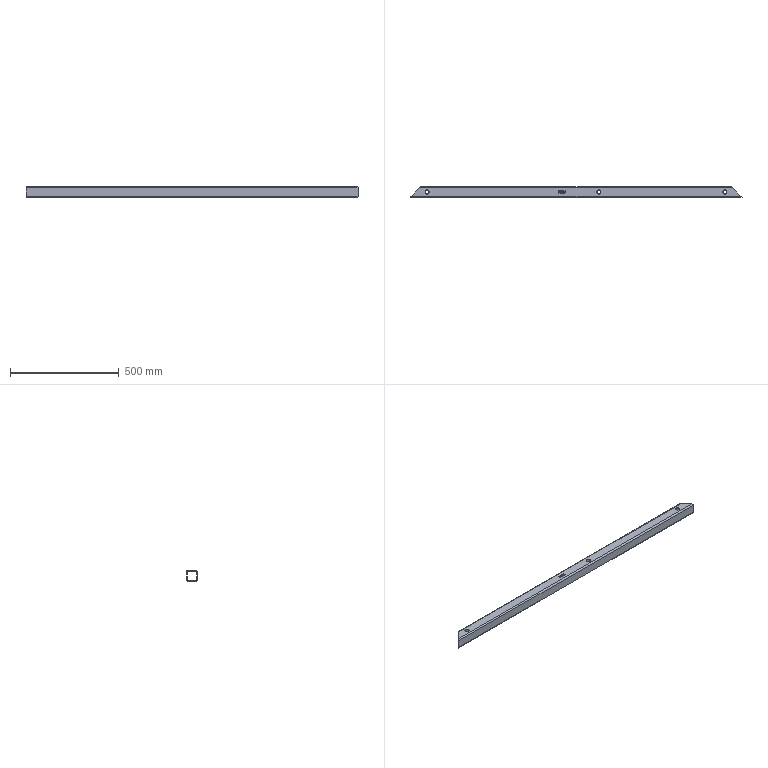Part | SolidWorks | features BaseBody 1 | 1 solid | 118 faces | box 1527 x 50 x 50 mm | volume 794723 mm3 | plane 68 | spline 30 | cylinder 20 | commonest cylinder face diameters 18 x6 18.8 x6 6 x4 12 x4